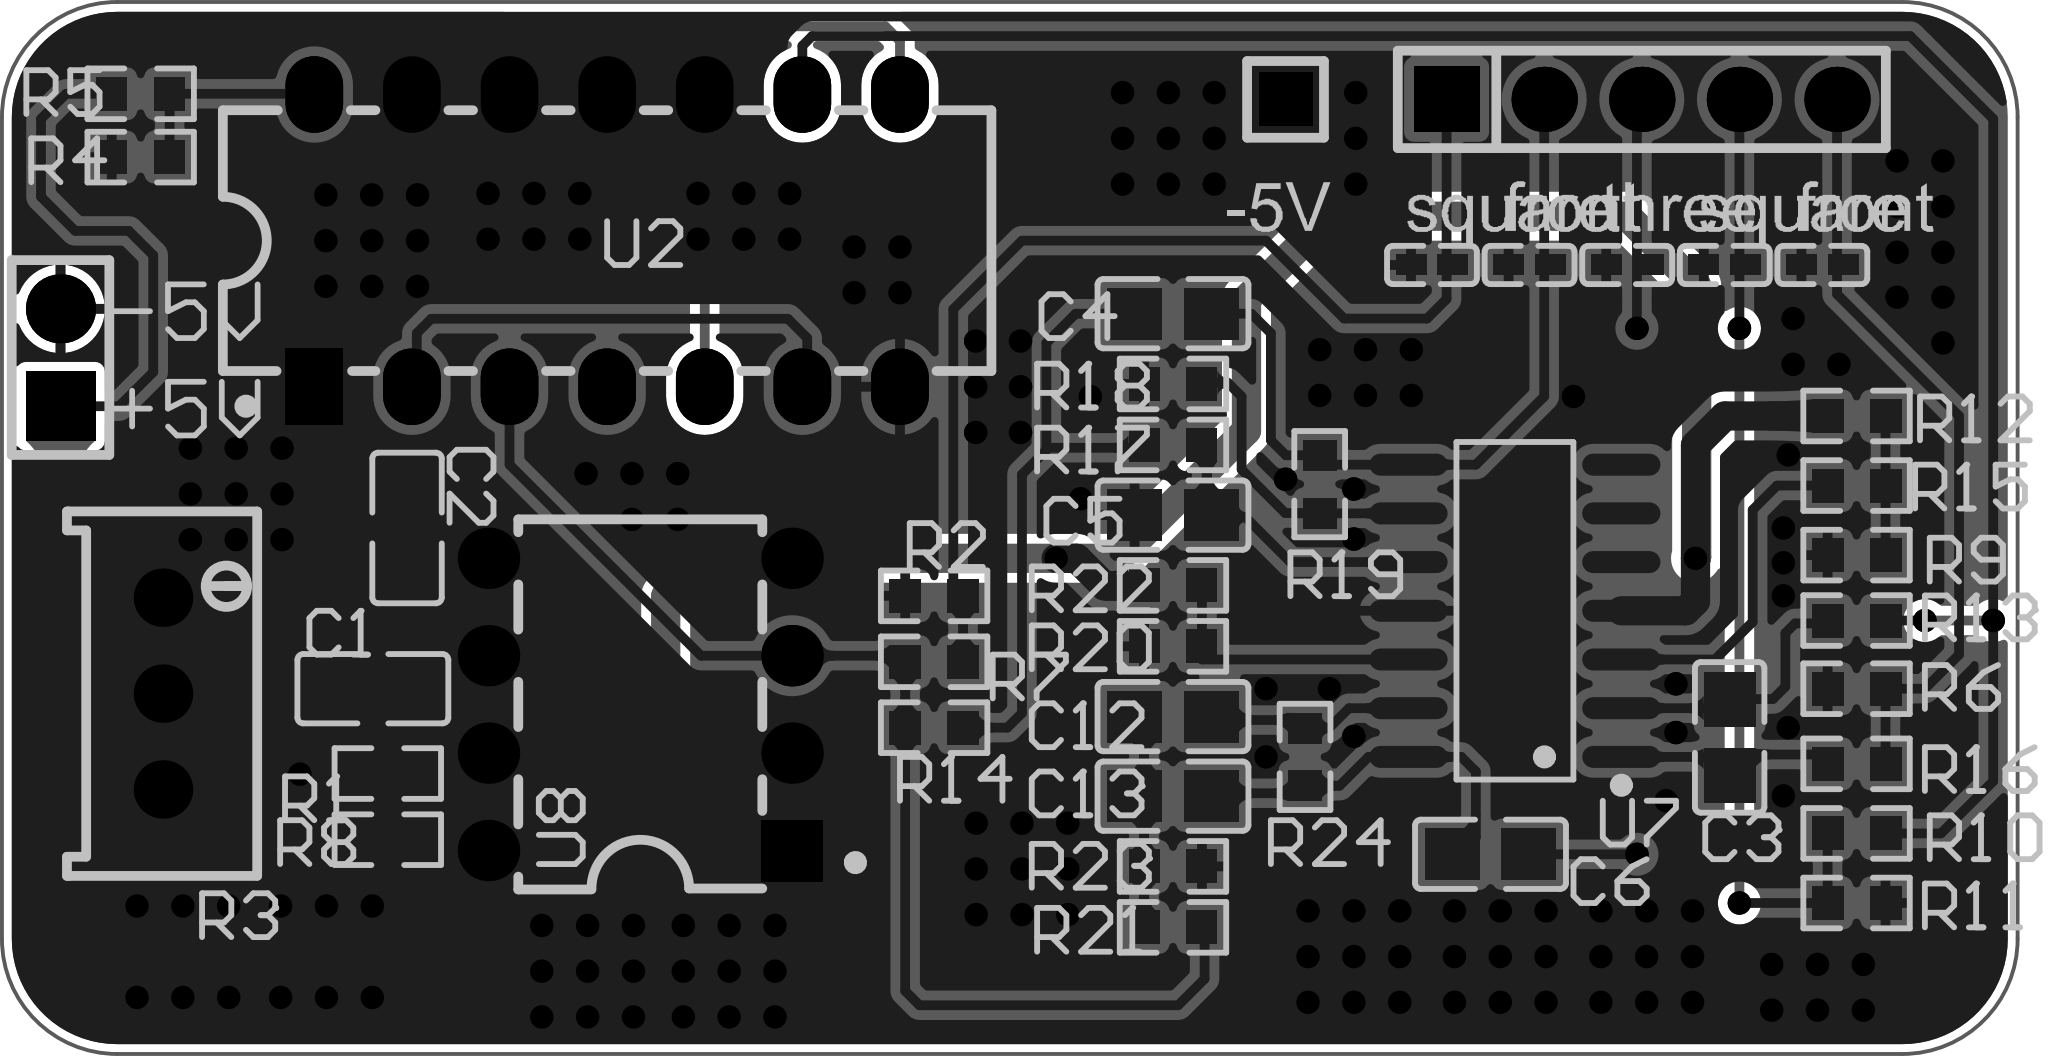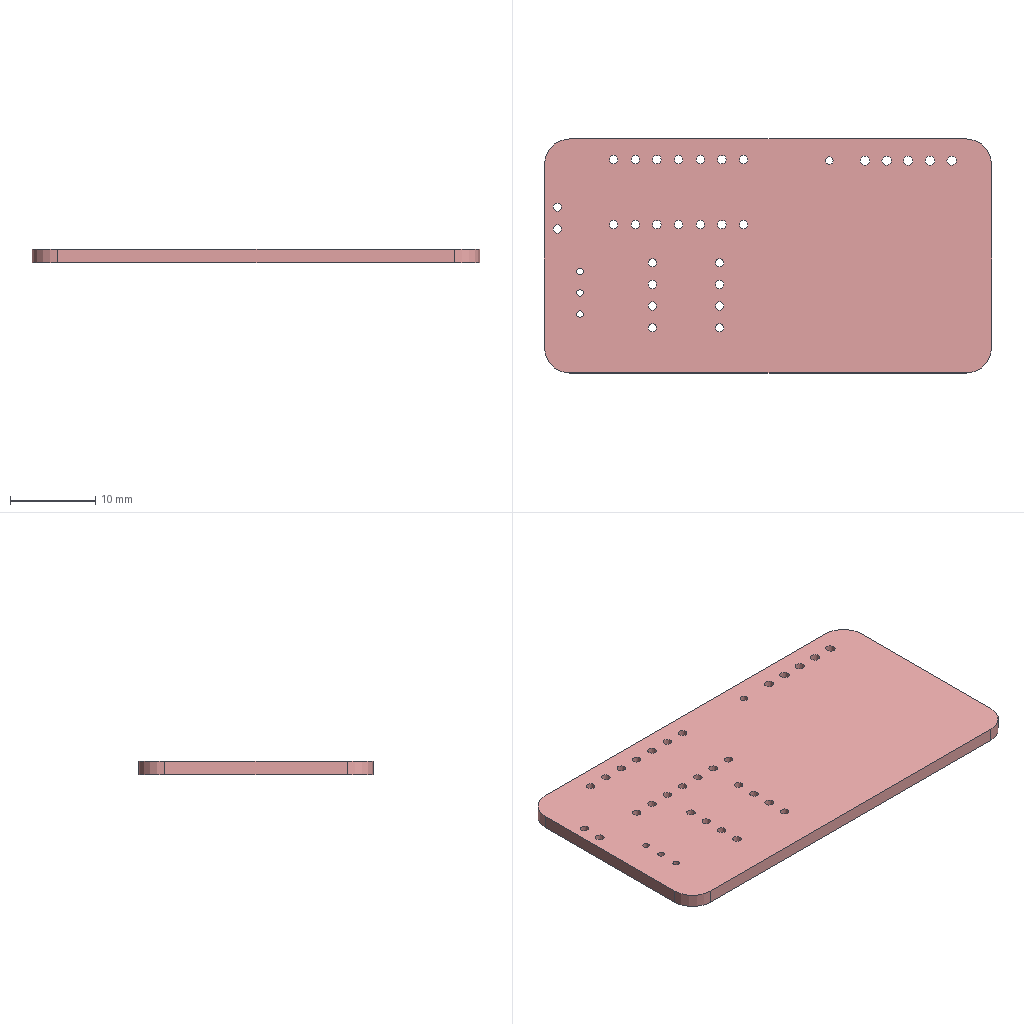Circuit board layout | Altium Designer | box 52.5 x 27.4 x 1.6 mm
Layer stack:
# Altium Designer layer stack of  (unit mm; dielectric type: 0 none, 1 core, 2 prepreg, 3 surface material)
index,name,kind,layer,copper_thickness_mm,dielectric_type,dielectric_thickness_mm,dielectric_material,dielectric_constant
0,Top Paste Mask Layer,other,,,,,,
1,Top Silkscreen Layer,other,,,,,,
2,Top Solder Mask Layer,dielectric,,,3,0.01,,3.3
3,Top Layer,copper,Top Layer,0.035,,,,
4,Dielectric1,dielectric,,,3,1.51,FR4,4.5
5,Bottom Layer,copper,Bottom Layer,0.035,,,,
6,Bottom Solder Mask Layer,dielectric,,,3,0.01,,3.3
7,Bottom Silkscreen Layer,other,,,,,,
8,Bottom Paste Mask Layer,other,,,,,,
# drill layer pairs: low layer,high layer
drill_pair,Top Layer,Bottom Layer
Part placement:
Designator,Comment,Layer,Footprint,Center-X(mm),Center-Y(mm),Rotation
H2,,TopLayer,HDR-TH_2P-P2.54-V-M-1,79.629,97.536,90
R1,510,TopLayer,R0603,88.146,86.688,180
R2,60,TopLayer,R0603,102.362,91.321,0
R4,1K,TopLayer,R0603,81.715,102.762,0
R5,1K,TopLayer,R0603,81.715,104.413,180
R6,200,TopLayer,R0603,126.365,88.9,0
R7,540,TopLayer,R0603,102.362,89.602,180
R8,12k,TopLayer,R0603,88.146,84.963,0
R9,100,TopLayer,R0603,126.365,92.383,180
R10,480,TopLayer,R0603,126.365,85.126,0
R11,120,TopLayer,R0603,126.365,83.312,180
R12,300,TopLayer,R0603,126.365,96.012,0
R13,1.8K,TopLayer,R0603,126.365,90.678,0
R14,10k,TopLayer,R0603,102.362,87.884,180
R15,1K,TopLayer,R0603,126.365,94.198,0
R16,400,TopLayer,R0603,126.365,86.941,180
R17,16.5k,TopLayer,R0603,108.577,95.258,180
R18,3.6k,TopLayer,R0603,108.577,96.847,180
R19,720,TopLayer,R0603,112.395,94.234,270
R20,1.35k,TopLayer,R0603,108.577,90.005,180
R21,41k,TopLayer,R0603,108.577,82.677,0
R22,1k,TopLayer,R0603,108.577,91.594,0
R23,50,TopLayer,R0603,108.577,84.266,0
R24,90k,TopLayer,R0603,112.014,87.122,270
U2,SN74LS74AN,TopLayer,PDIP-14_L19.5-W6.7-P2.54-LS7.9-BL,93.853,100.584,0
U7,LM324AD,TopLayer,SOIC-14_L8.7-W3.9-P1.27-LS6.0-BL,117.475,90.932,90
R3,24K,TopLayer,R_3296,82.296,88.773,270
U8,NE555PE4,TopLayer,PDIP-8_L9.6-W6.4-P2.54-LS7.9-BL-1,94.716,88.49,90
H3,,TopLayer,HDR-TH_5P-P2.54-V-M,120.777,104.267,0
H4,,TopLayer,HDR-TH_1P-V-M_XKB_X4611WV-01I-C28D40,111.506,104.267,0
C14,220nF,TopLayer,C0402,115.316,99.949,0
C14,220nF,TopLayer,C0402,117.856,99.949,0
C14,220nF,TopLayer,C0402,120.396,99.949,0
C14,220nF,TopLayer,C0402,122.936,99.949,0
C14,220nF,TopLayer,C0402,125.476,99.949,0
C1,1nF,TopLayer,C0805,87.757,88.9,180
C2,0.01uF,TopLayer,C0805,88.646,93.091,270
C3,10nF,TopLayer,C0805,123.063,87.63,90
C4,1nF,TopLayer,C0805,108.577,98.679,0
C5,1nF,TopLayer,C0805,108.577,93.426,0
C6,1nF,TopLayer,C0805,116.84,84.582,180
C12,0.11nF,TopLayer,C0805,108.577,88.173,180
C13,0.1nF,TopLayer,C0805,108.577,86.098,180
Pad and via stacks:
# Altium Designer via and pad stacks of  (unit mm). Each distinct definition once, with the count of objects using it.
# via: kind,start_layer,end_layer,hole_mm,diameter_mm,mode(0 simple;1 top-mid-bottom;2 full stack),diameter_per_layer,count,example_net
# pad: kind,layer,hole_mm,hole_type(0 round;1 square;2 slot),plating,top_size,top_shape(1 round;2 rect;3 octagon;9 rounded rect),mid_size,bottom_size,mode,footprint,size_per_layer,count,example
pad,Multi-Layer,1,0,plated,1.8x1.8,1,1.8x1.8,1.8x1.8,0,HDR-TH_2P-P2.54-V-M-1,,1,H2.2
pad,Multi-Layer,1,0,plated,1.8x1.8,2,1.8x1.8,1.8x1.8,0,HDR-TH_2P-P2.54-V-M-1,,1,H2.1
pad,Multi-Layer,1,0,plated,2x1.5,1,2x1.5,2x1.5,0,PDIP-14_L19.5-W6.7-P2.54-LS7.9-BL,,13,U2.8
pad,Multi-Layer,1,0,plated,2x1.5,2,2x1.5,2x1.5,0,PDIP-14_L19.5-W6.7-P2.54-LS7.9-BL,,1,U2.1
pad,Multi-Layer,0.762,0,plated,1.524x1.524,1,1.524x1.524,1.524x1.524,0,R_3296,,3,R3.2
pad,Multi-Layer,1,0,plated,1.6x1.6,1,1.6x1.6,1.6x1.6,0,PDIP-8_L9.6-W6.4-P2.54-LS7.9-BL-1,,7,U8.8
pad,Multi-Layer,1,0,plated,1.6x1.6,2,1.6x1.6,1.6x1.6,0,PDIP-8_L9.6-W6.4-P2.54-LS7.9-BL-1,,1,U8.1
pad,Multi-Layer,1.1,0,plated,1.7x1.7,2,1.7x1.7,1.7x1.7,0,HDR-TH_5P-P2.54-V-M,,1,H3.1
pad,Multi-Layer,1.1,0,plated,1.7x1.7,1,1.7x1.7,1.7x1.7,0,HDR-TH_5P-P2.54-V-M,,4,H3.2
pad,Multi-Layer,0.9,0,plated,1.4x1.4,2,1.4x1.4,1.4x1.4,0,HDR-TH_1P-V-M_XKB_X4611WV-01I-C28D40,,1,H4.1
pad,Top Layer,0,0,plated,0.8065x0.864,2,0.8065x0.864,0.8065x0.864,0,R0603,,46,R1.2
pad,Top Layer,0,0,plated,0.574x2.038,1,0.574x2.038,0.574x2.038,0,SOIC-14_L8.7-W3.9-P1.27-LS6.0-BL,,14,U7.1
pad,Top Layer,0,0,plated,0.7901x0.54,2,0.7901x0.54,0.7901x0.54,0,C0402,,10,C14.2
pad,Top Layer,0,0,plated,1.41x1.35,2,1.41x1.35,1.41x1.35,0,C0805,,16,C1.2
via,Top Layer,Bottom Layer,0.3048,0.61,0,,173,VCC
via,Top Layer,Bottom Layer,0.3048,0.6096,0,,2,VCC
Copper pours:
name,layer,net,type(0 solid;1 hatched;2 none)
Bottom Layer-GND,Bottom Layer,GND,0
Top Layer-GND,Top Layer,GND,0